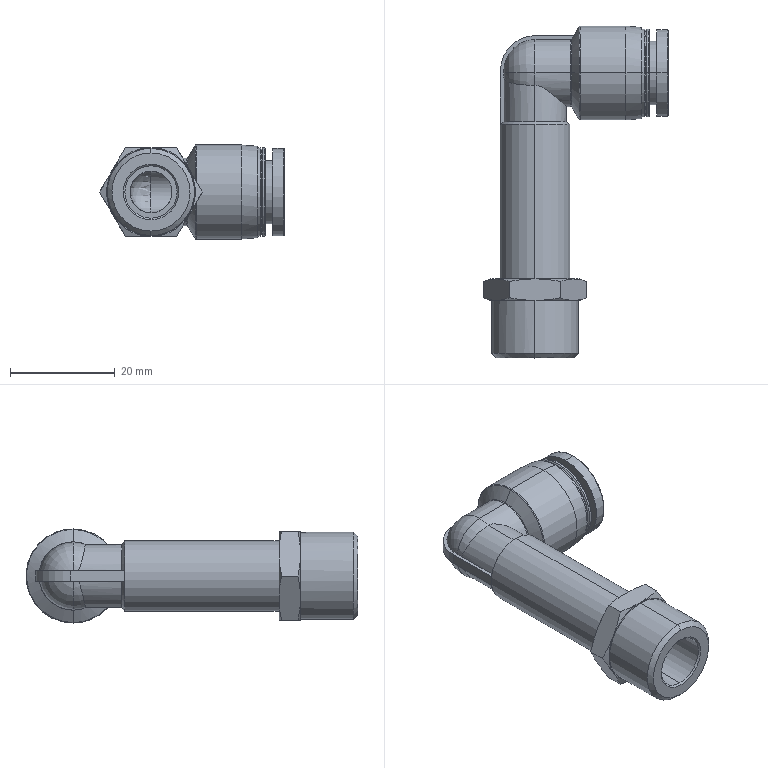Part | SolidWorks | features BaseBody 1 | 1 solid | 94 faces | box 35.315 x 63.5 x 18 mm | volume 9000 mm3 | cylinder 29 | cone 28 | plane 19 | torus 17 | sphere 1 | commonest cylinder face diameters 8 x4 10 x4 16.9 x4 12 x3 12.9 x3 13.4 x3